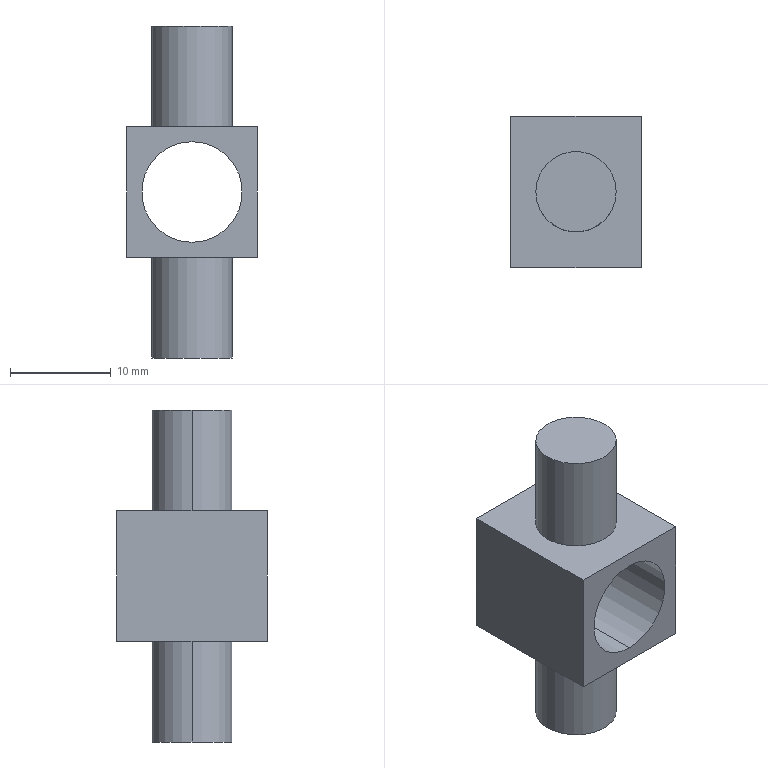Part | SolidWorks | features Extrusion 1, ICE 1, MirrorPattern 1 | 1 solid | 14 faces | box 13 x 15 x 33 mm | volume 2362 mm3 | plane 8 | cylinder 6 | commonest cylinder face diameters 8 x4 10 x2
STEP:
#1=CARTESIAN_POINT('',(4.,0.,-16.5));
#2=VERTEX_POINT('',#1);
#3=CARTESIAN_POINT('',(-4.,0.,-16.5));
#4=VERTEX_POINT('',#3);
#5=CARTESIAN_POINT('',(0.,0.,-16.5));
#6=DIRECTION('',(0.,0.,1.));
#7=DIRECTION('',(1.,0.,0.));
#8=AXIS2_PLACEMENT_3D('',#5,#6,#7);
#9=CIRCLE('',#8,4.);
#10=EDGE_CURVE('',#2,#4,#9,.T.);
#11=ORIENTED_EDGE('',*,*,#10,.T.);
#12=CARTESIAN_POINT('',(-4.,0.,-6.5));
#13=VERTEX_POINT('',#12);
#14=CARTESIAN_POINT('',(-4.,0.,-16.5));
#15=DIRECTION('',(0.,0.,1.));
#16=VECTOR('',#15,1000.);
#17=LINE('',#14,#16);
#18=EDGE_CURVE('',#4,#13,#17,.T.);
#19=ORIENTED_EDGE('',*,*,#18,.T.);
#20=CARTESIAN_POINT('',(4.,0.,-6.5));
#21=VERTEX_POINT('',#20);
#22=CARTESIAN_POINT('',(0.,0.,-6.5));
#23=DIRECTION('',(0.,0.,1.));
#24=DIRECTION('',(1.,0.,0.));
#25=AXIS2_PLACEMENT_3D('',#22,#23,#24);
#26=CIRCLE('',#25,4.);
#27=EDGE_CURVE('',#21,#13,#26,.T.);
#28=ORIENTED_EDGE('',*,*,#27,.F.);
#29=CARTESIAN_POINT('',(4.,0.,-16.5));
#30=DIRECTION('',(0.,0.,1.));
#31=VECTOR('',#30,1000.);
#32=LINE('',#29,#31);
#33=EDGE_CURVE('',#2,#21,#32,.T.);
#34=ORIENTED_EDGE('',*,*,#33,.F.);
#35=EDGE_LOOP('',(#11,#19,#28,#34));
#36=FACE_OUTER_BOUND('',#35,.T.);
#37=CARTESIAN_POINT('',(0.,0.,-16.5));
#38=DIRECTION('',(0.,0.,1.));
#39=DIRECTION('',(1.,0.,0.));
#40=AXIS2_PLACEMENT_3D('',#37,#38,#39);
#41=CYLINDRICAL_SURFACE('',#40,4.);
#42=ADVANCED_FACE('',(#36),#41,.T.);
#43=CARTESIAN_POINT('',(4.,0.,16.5));
#44=VERTEX_POINT('',#43);
#45=CARTESIAN_POINT('',(-4.,0.,16.5));
#46=VERTEX_POINT('',#45);
#47=CARTESIAN_POINT('',(0.,0.,16.5));
#48=DIRECTION('',(0.,0.,1.));
#49=DIRECTION('',(1.,0.,0.));
#50=AXIS2_PLACEMENT_3D('',#47,#48,#49);
#51=CIRCLE('',#50,4.);
#52=EDGE_CURVE('',#44,#46,#51,.T.);
#53=ORIENTED_EDGE('',*,*,#52,.F.);
#54=CARTESIAN_POINT('',(4.,0.,6.5));
#55=VERTEX_POINT('',#54);
#56=CARTESIAN_POINT('',(4.,0.,16.5));
#57=DIRECTION('',(0.,0.,-1.));
#58=VECTOR('',#57,1000.);
#59=LINE('',#56,#58);
#60=EDGE_CURVE('',#44,#55,#59,.T.);
#61=ORIENTED_EDGE('',*,*,#60,.T.);
#62=CARTESIAN_POINT('',(-4.,0.,6.5));
#63=VERTEX_POINT('',#62);
#64=CARTESIAN_POINT('',(0.,0.,6.5));
#65=DIRECTION('',(0.,0.,1.));
#66=DIRECTION('',(1.,0.,0.));
#67=AXIS2_PLACEMENT_3D('',#64,#65,#66);
#68=CIRCLE('',#67,4.);
#69=EDGE_CURVE('',#55,#63,#68,.T.);
#70=ORIENTED_EDGE('',*,*,#69,.T.);
#71=CARTESIAN_POINT('',(-4.,0.,16.5));
#72=DIRECTION('',(0.,0.,-1.));
#73=VECTOR('',#72,1000.);
#74=LINE('',#71,#73);
#75=EDGE_CURVE('',#46,#63,#74,.T.);
#76=ORIENTED_EDGE('',*,*,#75,.F.);
#77=EDGE_LOOP('',(#53,#61,#70,#76));
#78=FACE_OUTER_BOUND('',#77,.T.);
#79=CARTESIAN_POINT('',(0.,0.,16.5));
#80=DIRECTION('',(0.,0.,-1.));
#81=DIRECTION('',(-1.,0.,0.));
#82=AXIS2_PLACEMENT_3D('',#79,#80,#81);
#83=CYLINDRICAL_SURFACE('',#82,4.);
#84=ADVANCED_FACE('',(#78),#83,.T.);
#85=CARTESIAN_POINT('',(0.,7.5,-5.));
#86=VERTEX_POINT('',#85);
#87=CARTESIAN_POINT('',(0.,7.5,5.));
#88=VERTEX_POINT('',#87);
#89=CARTESIAN_POINT('',(0.,7.5,0.));
#90=DIRECTION('',(0.,1.,0.));
#91=DIRECTION('',(0.,0.,1.));
#92=AXIS2_PLACEMENT_3D('',#89,#90,#91);
#93=CIRCLE('',#92,5.);
#94=EDGE_CURVE('',#86,#88,#93,.T.);
#95=ORIENTED_EDGE('',*,*,#94,.T.);
#96=CARTESIAN_POINT('',(0.,-7.5,5.));
#97=VERTEX_POINT('',#96);
#98=CARTESIAN_POINT('',(0.,7.5,5.));
#99=DIRECTION('',(0.,-1.,0.));
#100=VECTOR('',#99,1000.);
#101=LINE('',#98,#100);
#102=EDGE_CURVE('',#88,#97,#101,.T.);
#103=ORIENTED_EDGE('',*,*,#102,.T.);
#104=CARTESIAN_POINT('',(0.,-7.5,-5.));
#105=VERTEX_POINT('',#104);
#106=CARTESIAN_POINT('',(0.,-7.5,0.));
#107=DIRECTION('',(0.,1.,0.));
#108=DIRECTION('',(0.,0.,1.));
#109=AXIS2_PLACEMENT_3D('',#106,#107,#108);
#110=CIRCLE('',#109,5.);
#111=EDGE_CURVE('',#105,#97,#110,.T.);
#112=ORIENTED_EDGE('',*,*,#111,.F.);
#113=CARTESIAN_POINT('',(0.,7.5,-5.));
#114=DIRECTION('',(0.,-1.,0.));
#115=VECTOR('',#114,1000.);
#116=LINE('',#113,#115);
#117=EDGE_CURVE('',#86,#105,#116,.T.);
#118=ORIENTED_EDGE('',*,*,#117,.F.);
#119=EDGE_LOOP('',(#95,#103,#112,#118));
#120=FACE_OUTER_BOUND('',#119,.T.);
#121=CARTESIAN_POINT('',(0.,7.5,0.));
#122=DIRECTION('',(0.,-1.,0.));
#123=DIRECTION('',(0.,0.,-1.));
#124=AXIS2_PLACEMENT_3D('',#121,#122,#123);
#125=CYLINDRICAL_SURFACE('',#124,5.);
#126=ADVANCED_FACE('',(#120),#125,.F.);
#127=CARTESIAN_POINT('',(6.5,7.5,6.5));
#128=VERTEX_POINT('',#127);
#129=CARTESIAN_POINT('',(6.5,7.5,-6.5));
#130=VERTEX_POINT('',#129);
#131=CARTESIAN_POINT('',(6.5,7.5,6.5));
#132=DIRECTION('',(0.,0.,-1.));
#133=VECTOR('',#132,1000.);
#134=LINE('',#131,#133);
#135=EDGE_CURVE('',#128,#130,#134,.T.);
#136=ORIENTED_EDGE('',*,*,#135,.T.);
#137=CARTESIAN_POINT('',(-6.5,7.5,-6.5));
#138=VERTEX_POINT('',#137);
#139=CARTESIAN_POINT('',(-6.5,7.5,-6.5));
#140=DIRECTION('',(-1.,0.,0.));
#141=VECTOR('',#140,1000.);
#142=LINE('',#139,#141);
#143=EDGE_CURVE('',#130,#138,#142,.T.);
#144=ORIENTED_EDGE('',*,*,#143,.T.);
#145=CARTESIAN_POINT('',(-6.5,7.5,6.5));
#146=VERTEX_POINT('',#145);
#147=CARTESIAN_POINT('',(-6.5,7.5,6.5));
#148=DIRECTION('',(0.,0.,1.));
#149=VECTOR('',#148,1000.);
#150=LINE('',#147,#149);
#151=EDGE_CURVE('',#138,#146,#150,.T.);
#152=ORIENTED_EDGE('',*,*,#151,.T.);
#153=CARTESIAN_POINT('',(-6.5,7.5,6.5));
#154=DIRECTION('',(1.,0.,0.));
#155=VECTOR('',#154,1000.);
#156=LINE('',#153,#155);
#157=EDGE_CURVE('',#146,#128,#156,.T.);
#158=ORIENTED_EDGE('',*,*,#157,.T.);
#159=EDGE_LOOP('',(#136,#144,#152,#158));
#160=FACE_OUTER_BOUND('',#159,.T.);
#161=ORIENTED_EDGE('',*,*,#94,.F.);
#162=CARTESIAN_POINT('',(0.,7.5,0.));
#163=DIRECTION('',(0.,1.,0.));
#164=DIRECTION('',(0.,0.,1.));
#165=AXIS2_PLACEMENT_3D('',#162,#163,#164);
#166=CIRCLE('',#165,5.);
#167=EDGE_CURVE('',#88,#86,#166,.T.);
#168=ORIENTED_EDGE('',*,*,#167,.F.);
#169=EDGE_LOOP('',(#161,#168));
#170=FACE_BOUND('',#169,.T.);
#171=CARTESIAN_POINT('',(0.,7.5,0.));
#172=DIRECTION('',(0.,-1.,0.));
#173=DIRECTION('',(0.,0.,-1.));
#174=AXIS2_PLACEMENT_3D('',#171,#172,#173);
#175=PLANE('',#174);
#176=ADVANCED_FACE('',(#160,#170),#175,.F.);
#177=CARTESIAN_POINT('',(6.5,-7.5,6.5));
#178=VERTEX_POINT('',#177);
#179=CARTESIAN_POINT('',(6.5,-7.5,-6.5));
#180=VERTEX_POINT('',#179);
#181=CARTESIAN_POINT('',(6.5,-7.5,6.5));
#182=DIRECTION('',(0.,0.,-1.));
#183=VECTOR('',#182,1000.);
#184=LINE('',#181,#183);
#185=EDGE_CURVE('',#178,#180,#184,.T.);
#186=ORIENTED_EDGE('',*,*,#185,.F.);
#187=CARTESIAN_POINT('',(-6.5,-7.5,6.5));
#188=VERTEX_POINT('',#187);
#189=CARTESIAN_POINT('',(-6.5,-7.5,6.5));
#190=DIRECTION('',(1.,0.,0.));
#191=VECTOR('',#190,1000.);
#192=LINE('',#189,#191);
#193=EDGE_CURVE('',#188,#178,#192,.T.);
#194=ORIENTED_EDGE('',*,*,#193,.F.);
#195=CARTESIAN_POINT('',(-6.5,-7.5,-6.5));
#196=VERTEX_POINT('',#195);
#197=CARTESIAN_POINT('',(-6.5,-7.5,6.5));
#198=DIRECTION('',(0.,0.,1.));
#199=VECTOR('',#198,1000.);
#200=LINE('',#197,#199);
#201=EDGE_CURVE('',#196,#188,#200,.T.);
#202=ORIENTED_EDGE('',*,*,#201,.F.);
#203=CARTESIAN_POINT('',(-6.5,-7.5,-6.5));
#204=DIRECTION('',(-1.,0.,0.));
#205=VECTOR('',#204,1000.);
#206=LINE('',#203,#205);
#207=EDGE_CURVE('',#180,#196,#206,.T.);
#208=ORIENTED_EDGE('',*,*,#207,.F.);
#209=EDGE_LOOP('',(#186,#194,#202,#208));
#210=FACE_OUTER_BOUND('',#209,.T.);
#211=ORIENTED_EDGE('',*,*,#111,.T.);
#212=CARTESIAN_POINT('',(0.,-7.5,0.));
#213=DIRECTION('',(0.,1.,0.));
#214=DIRECTION('',(0.,0.,1.));
#215=AXIS2_PLACEMENT_3D('',#212,#213,#214);
#216=CIRCLE('',#215,5.);
#217=EDGE_CURVE('',#97,#105,#216,.T.);
#218=ORIENTED_EDGE('',*,*,#217,.T.);
#219=EDGE_LOOP('',(#211,#218));
#220=FACE_BOUND('',#219,.T.);
#221=CARTESIAN_POINT('',(0.,-7.5,0.));
#222=DIRECTION('',(0.,-1.,0.));
#223=DIRECTION('',(0.,0.,-1.));
#224=AXIS2_PLACEMENT_3D('',#221,#222,#223);
#225=PLANE('',#224);
#226=ADVANCED_FACE('',(#210,#220),#225,.T.);
#227=ORIENTED_EDGE('',*,*,#185,.T.);
#228=CARTESIAN_POINT('',(6.5,7.5,-6.5));
#229=DIRECTION('',(0.,-1.,0.));
#230=VECTOR('',#229,1000.);
#231=LINE('',#228,#230);
#232=EDGE_CURVE('',#130,#180,#231,.T.);
#233=ORIENTED_EDGE('',*,*,#232,.F.);
#234=ORIENTED_EDGE('',*,*,#135,.F.);
#235=CARTESIAN_POINT('',(6.5,7.5,6.5));
#236=DIRECTION('',(0.,-1.,0.));
#237=VECTOR('',#236,1000.);
#238=LINE('',#235,#237);
#239=EDGE_CURVE('',#128,#178,#238,.T.);
#240=ORIENTED_EDGE('',*,*,#239,.T.);
#241=EDGE_LOOP('',(#227,#233,#234,#240));
#242=FACE_OUTER_BOUND('',#241,.T.);
#243=CARTESIAN_POINT('',(6.5,7.5,6.5));
#244=DIRECTION('',(-1.,0.,0.));
#245=DIRECTION('',(0.,0.,1.));
#246=AXIS2_PLACEMENT_3D('',#243,#244,#245);
#247=PLANE('',#246);
#248=ADVANCED_FACE('',(#242),#247,.F.);
#249=ORIENTED_EDGE('',*,*,#27,.T.);
#250=CARTESIAN_POINT('',(0.,0.,-6.5));
#251=DIRECTION('',(0.,0.,1.));
#252=DIRECTION('',(1.,0.,0.));
#253=AXIS2_PLACEMENT_3D('',#250,#251,#252);
#254=CIRCLE('',#253,4.);
#255=EDGE_CURVE('',#13,#21,#254,.T.);
#256=ORIENTED_EDGE('',*,*,#255,.T.);
#257=EDGE_LOOP('',(#249,#256));
#258=FACE_BOUND('',#257,.T.);
#259=ORIENTED_EDGE('',*,*,#207,.T.);
#260=CARTESIAN_POINT('',(-6.5,7.5,-6.5));
#261=DIRECTION('',(0.,-1.,0.));
#262=VECTOR('',#261,1000.);
#263=LINE('',#260,#262);
#264=EDGE_CURVE('',#138,#196,#263,.T.);
#265=ORIENTED_EDGE('',*,*,#264,.F.);
#266=ORIENTED_EDGE('',*,*,#143,.F.);
#267=ORIENTED_EDGE('',*,*,#232,.T.);
#268=EDGE_LOOP('',(#259,#265,#266,#267));
#269=FACE_OUTER_BOUND('',#268,.T.);
#270=CARTESIAN_POINT('',(-6.5,7.5,-6.5));
#271=DIRECTION('',(0.,0.,1.));
#272=DIRECTION('',(1.,0.,0.));
#273=AXIS2_PLACEMENT_3D('',#270,#271,#272);
#274=PLANE('',#273);
#275=ADVANCED_FACE('',(#258,#269),#274,.F.);
#276=ORIENTED_EDGE('',*,*,#201,.T.);
#277=CARTESIAN_POINT('',(-6.5,7.5,6.5));
#278=DIRECTION('',(0.,-1.,0.));
#279=VECTOR('',#278,1000.);
#280=LINE('',#277,#279);
#281=EDGE_CURVE('',#146,#188,#280,.T.);
#282=ORIENTED_EDGE('',*,*,#281,.F.);
#283=ORIENTED_EDGE('',*,*,#151,.F.);
#284=ORIENTED_EDGE('',*,*,#264,.T.);
#285=EDGE_LOOP('',(#276,#282,#283,#284));
#286=FACE_OUTER_BOUND('',#285,.T.);
#287=CARTESIAN_POINT('',(-6.5,7.5,6.5));
#288=DIRECTION('',(1.,0.,0.));
#289=DIRECTION('',(0.,0.,-1.));
#290=AXIS2_PLACEMENT_3D('',#287,#288,#289);
#291=PLANE('',#290);
#292=ADVANCED_FACE('',(#286),#291,.F.);
#293=CARTESIAN_POINT('',(0.,0.,6.5));
#294=DIRECTION('',(0.,0.,1.));
#295=DIRECTION('',(1.,0.,0.));
#296=AXIS2_PLACEMENT_3D('',#293,#294,#295);
#297=CIRCLE('',#296,4.);
#298=EDGE_CURVE('',#63,#55,#297,.T.);
#299=ORIENTED_EDGE('',*,*,#298,.F.);
#300=ORIENTED_EDGE('',*,*,#69,.F.);
#301=EDGE_LOOP('',(#299,#300));
#302=FACE_BOUND('',#301,.T.);
#303=ORIENTED_EDGE('',*,*,#193,.T.);
#304=ORIENTED_EDGE('',*,*,#239,.F.);
#305=ORIENTED_EDGE('',*,*,#157,.F.);
#306=ORIENTED_EDGE('',*,*,#281,.T.);
#307=EDGE_LOOP('',(#303,#304,#305,#306));
#308=FACE_OUTER_BOUND('',#307,.T.);
#309=CARTESIAN_POINT('',(-6.5,7.5,6.5));
#310=DIRECTION('',(0.,0.,-1.));
#311=DIRECTION('',(-1.,0.,0.));
#312=AXIS2_PLACEMENT_3D('',#309,#310,#311);
#313=PLANE('',#312);
#314=ADVANCED_FACE('',(#302,#308),#313,.F.);
#315=ORIENTED_EDGE('',*,*,#102,.F.);
#316=ORIENTED_EDGE('',*,*,#167,.T.);
#317=ORIENTED_EDGE('',*,*,#117,.T.);
#318=ORIENTED_EDGE('',*,*,#217,.F.);
#319=EDGE_LOOP('',(#315,#316,#317,#318));
#320=FACE_OUTER_BOUND('',#319,.T.);
#321=CARTESIAN_POINT('',(0.,7.5,0.));
#322=DIRECTION('',(0.,-1.,0.));
#323=DIRECTION('',(0.,0.,-1.));
#324=AXIS2_PLACEMENT_3D('',#321,#322,#323);
#325=CYLINDRICAL_SURFACE('',#324,5.);
#326=ADVANCED_FACE('',(#320),#325,.F.);
#327=ORIENTED_EDGE('',*,*,#60,.F.);
#328=CARTESIAN_POINT('',(0.,0.,16.5));
#329=DIRECTION('',(0.,0.,1.));
#330=DIRECTION('',(1.,0.,0.));
#331=AXIS2_PLACEMENT_3D('',#328,#329,#330);
#332=CIRCLE('',#331,4.);
#333=EDGE_CURVE('',#46,#44,#332,.T.);
#334=ORIENTED_EDGE('',*,*,#333,.F.);
#335=ORIENTED_EDGE('',*,*,#75,.T.);
#336=ORIENTED_EDGE('',*,*,#298,.T.);
#337=EDGE_LOOP('',(#327,#334,#335,#336));
#338=FACE_OUTER_BOUND('',#337,.T.);
#339=CARTESIAN_POINT('',(0.,0.,16.5));
#340=DIRECTION('',(0.,0.,-1.));
#341=DIRECTION('',(-1.,0.,0.));
#342=AXIS2_PLACEMENT_3D('',#339,#340,#341);
#343=CYLINDRICAL_SURFACE('',#342,4.);
#344=ADVANCED_FACE('',(#338),#343,.T.);
#345=ORIENTED_EDGE('',*,*,#333,.T.);
#346=ORIENTED_EDGE('',*,*,#52,.T.);
#347=EDGE_LOOP('',(#345,#346));
#348=FACE_OUTER_BOUND('',#347,.T.);
#349=CARTESIAN_POINT('',(0.,0.,16.5));
#350=DIRECTION('',(0.,0.,1.));
#351=DIRECTION('',(1.,0.,0.));
#352=AXIS2_PLACEMENT_3D('',#349,#350,#351);
#353=PLANE('',#352);
#354=ADVANCED_FACE('',(#348),#353,.T.);
#355=ORIENTED_EDGE('',*,*,#18,.F.);
#356=CARTESIAN_POINT('',(0.,0.,-16.5));
#357=DIRECTION('',(0.,0.,1.));
#358=DIRECTION('',(1.,0.,0.));
#359=AXIS2_PLACEMENT_3D('',#356,#357,#358);
#360=CIRCLE('',#359,4.);
#361=EDGE_CURVE('',#4,#2,#360,.T.);
#362=ORIENTED_EDGE('',*,*,#361,.T.);
#363=ORIENTED_EDGE('',*,*,#33,.T.);
#364=ORIENTED_EDGE('',*,*,#255,.F.);
#365=EDGE_LOOP('',(#355,#362,#363,#364));
#366=FACE_OUTER_BOUND('',#365,.T.);
#367=CARTESIAN_POINT('',(0.,0.,-16.5));
#368=DIRECTION('',(0.,0.,1.));
#369=DIRECTION('',(1.,0.,0.));
#370=AXIS2_PLACEMENT_3D('',#367,#368,#369);
#371=CYLINDRICAL_SURFACE('',#370,4.);
#372=ADVANCED_FACE('',(#366),#371,.T.);
#373=ORIENTED_EDGE('',*,*,#10,.F.);
#374=ORIENTED_EDGE('',*,*,#361,.F.);
#375=EDGE_LOOP('',(#373,#374));
#376=FACE_OUTER_BOUND('',#375,.T.);
#377=CARTESIAN_POINT('',(0.,0.,-16.5));
#378=DIRECTION('',(0.,0.,-1.));
#379=DIRECTION('',(1.,0.,0.));
#380=AXIS2_PLACEMENT_3D('',#377,#378,#379);
#381=PLANE('',#380);
#382=ADVANCED_FACE('',(#376),#381,.T.);
#383=CLOSED_SHELL('',(#42,#84,#126,#176,#226,#248,#275,#292,#314,#326,#344,#354,#372,#382));
#384=MANIFOLD_SOLID_BREP('',#383);
#385=CARTESIAN_POINT('',(0.,0.,0.));
#386=DIRECTION('',(0.,0.,1.));
#387=DIRECTION('',(1.,0.,0.));
#388=AXIS2_PLACEMENT_3D('',#385,#386,#387);
#389=(LENGTH_UNIT()NAMED_UNIT(*)SI_UNIT(.MILLI.,.METRE.));
#390=UNCERTAINTY_MEASURE_WITH_UNIT(LENGTH_MEASURE(0.00001),#389,'','');
#391=(NAMED_UNIT(*)PLANE_ANGLE_UNIT()SI_UNIT($,.RADIAN.));
#392=(NAMED_UNIT(*)SI_UNIT($,.STERADIAN.)SOLID_ANGLE_UNIT());
#393=(GEOMETRIC_REPRESENTATION_CONTEXT(3)GLOBAL_UNCERTAINTY_ASSIGNED_CONTEXT((#390))GLOBAL_UNIT_ASSIGNED_CONTEXT((#389,#391,#392))REPRESENTATION_CONTEXT('',''));
#394=ADVANCED_BREP_SHAPE_REPRESENTATION('',(#384,#388),#393);